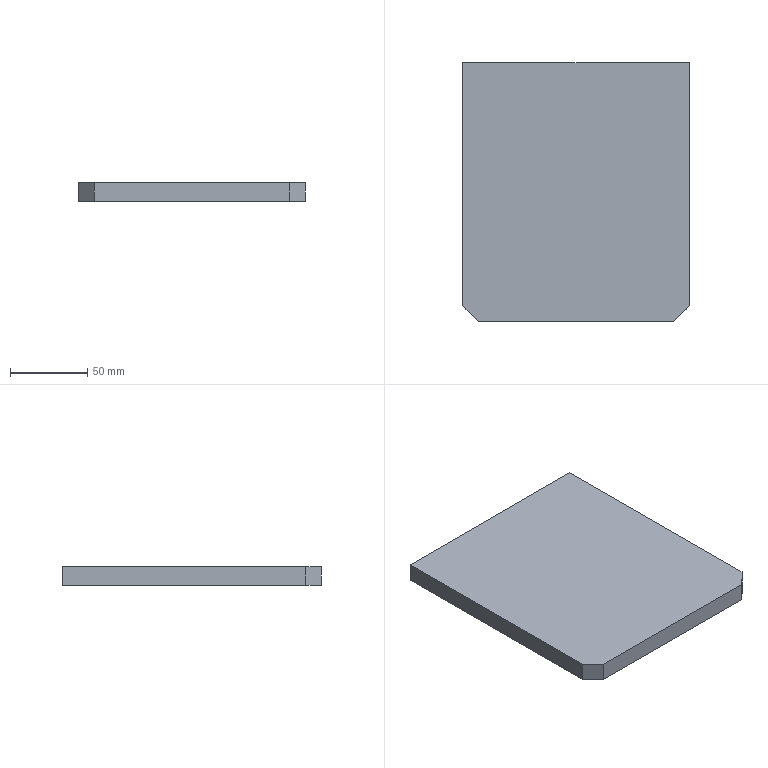Part | SolidWorks | features BaseBody 1 | 1 solid | 8 faces | box 146 x 167 x 12 mm | volume 291384 mm3 | plane 8
STEP:
#1=CARTESIAN_POINT('',(-73.,82.,6.));
#2=VERTEX_POINT('',#1);
#3=CARTESIAN_POINT('',(-73.,-75.,6.));
#4=VERTEX_POINT('',#3);
#5=CARTESIAN_POINT('',(-73.,85.,6.));
#6=DIRECTION('',(0.,-1.,0.));
#7=VECTOR('',#6,1000.);
#8=LINE('',#5,#7);
#9=EDGE_CURVE('',#2,#4,#8,.T.);
#10=ORIENTED_EDGE('',*,*,#9,.F.);
#11=CARTESIAN_POINT('',(-73.,82.,-6.));
#12=VERTEX_POINT('',#11);
#13=CARTESIAN_POINT('',(-73.,82.,6.));
#14=DIRECTION('',(0.,0.,-1.));
#15=VECTOR('',#14,1000.);
#16=LINE('',#13,#15);
#17=EDGE_CURVE('',#2,#12,#16,.T.);
#18=ORIENTED_EDGE('',*,*,#17,.T.);
#19=CARTESIAN_POINT('',(-73.,-75.,-6.));
#20=VERTEX_POINT('',#19);
#21=CARTESIAN_POINT('',(-73.,85.,-6.));
#22=DIRECTION('',(0.,-1.,0.));
#23=VECTOR('',#22,1000.);
#24=LINE('',#21,#23);
#25=EDGE_CURVE('',#12,#20,#24,.T.);
#26=ORIENTED_EDGE('',*,*,#25,.T.);
#27=CARTESIAN_POINT('',(-73.,-75.,6.));
#28=DIRECTION('',(0.,0.,-1.));
#29=VECTOR('',#28,1000.);
#30=LINE('',#27,#29);
#31=EDGE_CURVE('',#4,#20,#30,.T.);
#32=ORIENTED_EDGE('',*,*,#31,.F.);
#33=EDGE_LOOP('',(#10,#18,#26,#32));
#34=FACE_OUTER_BOUND('',#33,.T.);
#35=CARTESIAN_POINT('',(-73.,85.,6.));
#36=DIRECTION('',(1.,0.,0.));
#37=DIRECTION('',(0.,1.,0.));
#38=AXIS2_PLACEMENT_3D('',#35,#36,#37);
#39=PLANE('',#38);
#40=ADVANCED_FACE('',(#34),#39,.F.);
#41=CARTESIAN_POINT('',(-63.,-85.,-6.));
#42=VERTEX_POINT('',#41);
#43=CARTESIAN_POINT('',(-73.,-75.,-6.));
#44=DIRECTION('',(0.7071,-0.7071,0.));
#45=VECTOR('',#44,1000.);
#46=LINE('',#43,#45);
#47=EDGE_CURVE('',#20,#42,#46,.T.);
#48=ORIENTED_EDGE('',*,*,#47,.T.);
#49=CARTESIAN_POINT('',(-63.,-85.,6.));
#50=VERTEX_POINT('',#49);
#51=CARTESIAN_POINT('',(-63.,-85.,6.));
#52=DIRECTION('',(0.,0.,-1.));
#53=VECTOR('',#52,1000.);
#54=LINE('',#51,#53);
#55=EDGE_CURVE('',#50,#42,#54,.T.);
#56=ORIENTED_EDGE('',*,*,#55,.F.);
#57=CARTESIAN_POINT('',(-73.,-75.,6.));
#58=DIRECTION('',(0.7071,-0.7071,0.));
#59=VECTOR('',#58,1000.);
#60=LINE('',#57,#59);
#61=EDGE_CURVE('',#4,#50,#60,.T.);
#62=ORIENTED_EDGE('',*,*,#61,.F.);
#63=ORIENTED_EDGE('',*,*,#31,.T.);
#64=EDGE_LOOP('',(#48,#56,#62,#63));
#65=FACE_OUTER_BOUND('',#64,.T.);
#66=CARTESIAN_POINT('',(-73.,-75.,6.));
#67=DIRECTION('',(0.7071,0.7071,0.));
#68=DIRECTION('',(-0.7071,0.7071,0.));
#69=AXIS2_PLACEMENT_3D('',#66,#67,#68);
#70=PLANE('',#69);
#71=ADVANCED_FACE('',(#65),#70,.F.);
#72=CARTESIAN_POINT('',(63.,-85.,-6.));
#73=VERTEX_POINT('',#72);
#74=CARTESIAN_POINT('',(-63.,-85.,-6.));
#75=DIRECTION('',(1.,0.,0.));
#76=VECTOR('',#75,1000.);
#77=LINE('',#74,#76);
#78=EDGE_CURVE('',#42,#73,#77,.T.);
#79=ORIENTED_EDGE('',*,*,#78,.T.);
#80=CARTESIAN_POINT('',(63.,-85.,6.));
#81=VERTEX_POINT('',#80);
#82=CARTESIAN_POINT('',(63.,-85.,6.));
#83=DIRECTION('',(0.,0.,-1.));
#84=VECTOR('',#83,1000.);
#85=LINE('',#82,#84);
#86=EDGE_CURVE('',#81,#73,#85,.T.);
#87=ORIENTED_EDGE('',*,*,#86,.F.);
#88=CARTESIAN_POINT('',(-63.,-85.,6.));
#89=DIRECTION('',(1.,0.,0.));
#90=VECTOR('',#89,1000.);
#91=LINE('',#88,#90);
#92=EDGE_CURVE('',#50,#81,#91,.T.);
#93=ORIENTED_EDGE('',*,*,#92,.F.);
#94=ORIENTED_EDGE('',*,*,#55,.T.);
#95=EDGE_LOOP('',(#79,#87,#93,#94));
#96=FACE_OUTER_BOUND('',#95,.T.);
#97=CARTESIAN_POINT('',(-63.,-85.,6.));
#98=DIRECTION('',(0.,1.,0.));
#99=DIRECTION('',(0.,0.,1.));
#100=AXIS2_PLACEMENT_3D('',#97,#98,#99);
#101=PLANE('',#100);
#102=ADVANCED_FACE('',(#96),#101,.F.);
#103=CARTESIAN_POINT('',(73.,-75.,-6.));
#104=VERTEX_POINT('',#103);
#105=CARTESIAN_POINT('',(63.,-85.,-6.));
#106=DIRECTION('',(0.7071,0.7071,0.));
#107=VECTOR('',#106,1000.);
#108=LINE('',#105,#107);
#109=EDGE_CURVE('',#73,#104,#108,.T.);
#110=ORIENTED_EDGE('',*,*,#109,.T.);
#111=CARTESIAN_POINT('',(73.,-75.,6.));
#112=VERTEX_POINT('',#111);
#113=CARTESIAN_POINT('',(73.,-75.,6.));
#114=DIRECTION('',(0.,0.,-1.));
#115=VECTOR('',#114,1000.);
#116=LINE('',#113,#115);
#117=EDGE_CURVE('',#112,#104,#116,.T.);
#118=ORIENTED_EDGE('',*,*,#117,.F.);
#119=CARTESIAN_POINT('',(63.,-85.,6.));
#120=DIRECTION('',(0.7071,0.7071,0.));
#121=VECTOR('',#120,1000.);
#122=LINE('',#119,#121);
#123=EDGE_CURVE('',#81,#112,#122,.T.);
#124=ORIENTED_EDGE('',*,*,#123,.F.);
#125=ORIENTED_EDGE('',*,*,#86,.T.);
#126=EDGE_LOOP('',(#110,#118,#124,#125));
#127=FACE_OUTER_BOUND('',#126,.T.);
#128=CARTESIAN_POINT('',(63.,-85.,6.));
#129=DIRECTION('',(-0.7071,0.7071,0.));
#130=DIRECTION('',(-0.7071,-0.7071,0.));
#131=AXIS2_PLACEMENT_3D('',#128,#129,#130);
#132=PLANE('',#131);
#133=ADVANCED_FACE('',(#127),#132,.F.);
#134=CARTESIAN_POINT('',(73.,82.,-6.));
#135=VERTEX_POINT('',#134);
#136=CARTESIAN_POINT('',(73.,85.,-6.));
#137=DIRECTION('',(0.,1.,0.));
#138=VECTOR('',#137,1000.);
#139=LINE('',#136,#138);
#140=EDGE_CURVE('',#104,#135,#139,.T.);
#141=ORIENTED_EDGE('',*,*,#140,.T.);
#142=CARTESIAN_POINT('',(73.,82.,6.));
#143=VERTEX_POINT('',#142);
#144=CARTESIAN_POINT('',(73.,82.,6.));
#145=DIRECTION('',(0.,0.,1.));
#146=VECTOR('',#145,1000.);
#147=LINE('',#144,#146);
#148=EDGE_CURVE('',#135,#143,#147,.T.);
#149=ORIENTED_EDGE('',*,*,#148,.T.);
#150=CARTESIAN_POINT('',(73.,85.,6.));
#151=DIRECTION('',(0.,1.,0.));
#152=VECTOR('',#151,1000.);
#153=LINE('',#150,#152);
#154=EDGE_CURVE('',#112,#143,#153,.T.);
#155=ORIENTED_EDGE('',*,*,#154,.F.);
#156=ORIENTED_EDGE('',*,*,#117,.T.);
#157=EDGE_LOOP('',(#141,#149,#155,#156));
#158=FACE_OUTER_BOUND('',#157,.T.);
#159=CARTESIAN_POINT('',(73.,85.,6.));
#160=DIRECTION('',(-1.,0.,0.));
#161=DIRECTION('',(0.,0.,1.));
#162=AXIS2_PLACEMENT_3D('',#159,#160,#161);
#163=PLANE('',#162);
#164=ADVANCED_FACE('',(#158),#163,.F.);
#165=CARTESIAN_POINT('',(0.,82.,6.));
#166=DIRECTION('',(1.,0.,0.));
#167=VECTOR('',#166,1000.);
#168=LINE('',#165,#167);
#169=EDGE_CURVE('',#2,#143,#168,.T.);
#170=ORIENTED_EDGE('',*,*,#169,.F.);
#171=ORIENTED_EDGE('',*,*,#9,.T.);
#172=ORIENTED_EDGE('',*,*,#61,.T.);
#173=ORIENTED_EDGE('',*,*,#92,.T.);
#174=ORIENTED_EDGE('',*,*,#123,.T.);
#175=ORIENTED_EDGE('',*,*,#154,.T.);
#176=EDGE_LOOP('',(#170,#171,#172,#173,#174,#175));
#177=FACE_OUTER_BOUND('',#176,.T.);
#178=CARTESIAN_POINT('',(0.,0.,6.));
#179=DIRECTION('',(0.,0.,1.));
#180=DIRECTION('',(1.,0.,0.));
#181=AXIS2_PLACEMENT_3D('',#178,#179,#180);
#182=PLANE('',#181);
#183=ADVANCED_FACE('',(#177),#182,.T.);
#184=ORIENTED_EDGE('',*,*,#25,.F.);
#185=CARTESIAN_POINT('',(0.,82.,-6.));
#186=DIRECTION('',(1.,0.,0.));
#187=VECTOR('',#186,1000.);
#188=LINE('',#185,#187);
#189=EDGE_CURVE('',#12,#135,#188,.T.);
#190=ORIENTED_EDGE('',*,*,#189,.T.);
#191=ORIENTED_EDGE('',*,*,#140,.F.);
#192=ORIENTED_EDGE('',*,*,#109,.F.);
#193=ORIENTED_EDGE('',*,*,#78,.F.);
#194=ORIENTED_EDGE('',*,*,#47,.F.);
#195=EDGE_LOOP('',(#184,#190,#191,#192,#193,#194));
#196=FACE_OUTER_BOUND('',#195,.T.);
#197=CARTESIAN_POINT('',(0.,0.,-6.));
#198=DIRECTION('',(0.,0.,1.));
#199=DIRECTION('',(1.,0.,0.));
#200=AXIS2_PLACEMENT_3D('',#197,#198,#199);
#201=PLANE('',#200);
#202=ADVANCED_FACE('',(#196),#201,.F.);
#203=ORIENTED_EDGE('',*,*,#169,.T.);
#204=ORIENTED_EDGE('',*,*,#148,.F.);
#205=ORIENTED_EDGE('',*,*,#189,.F.);
#206=ORIENTED_EDGE('',*,*,#17,.F.);
#207=EDGE_LOOP('',(#203,#204,#205,#206));
#208=FACE_OUTER_BOUND('',#207,.T.);
#209=CARTESIAN_POINT('',(0.,82.,589.));
#210=DIRECTION('',(0.,-1.,0.));
#211=DIRECTION('',(1.,0.,0.));
#212=AXIS2_PLACEMENT_3D('',#209,#210,#211);
#213=PLANE('',#212);
#214=ADVANCED_FACE('',(#208),#213,.F.);
#215=CLOSED_SHELL('',(#40,#71,#102,#133,#164,#183,#202,#214));
#216=MANIFOLD_SOLID_BREP('',#215);
#217=CARTESIAN_POINT('',(0.,0.,0.));
#218=DIRECTION('',(0.,0.,1.));
#219=DIRECTION('',(1.,0.,0.));
#220=AXIS2_PLACEMENT_3D('',#217,#218,#219);
#221=(LENGTH_UNIT()NAMED_UNIT(*)SI_UNIT(.MILLI.,.METRE.));
#222=UNCERTAINTY_MEASURE_WITH_UNIT(LENGTH_MEASURE(0.00001),#221,'','');
#223=(NAMED_UNIT(*)PLANE_ANGLE_UNIT()SI_UNIT($,.RADIAN.));
#224=(NAMED_UNIT(*)SI_UNIT($,.STERADIAN.)SOLID_ANGLE_UNIT());
#225=(GEOMETRIC_REPRESENTATION_CONTEXT(3)GLOBAL_UNCERTAINTY_ASSIGNED_CONTEXT((#222))GLOBAL_UNIT_ASSIGNED_CONTEXT((#221,#223,#224))REPRESENTATION_CONTEXT('',''));
#226=ADVANCED_BREP_SHAPE_REPRESENTATION('',(#216,#220),#225);